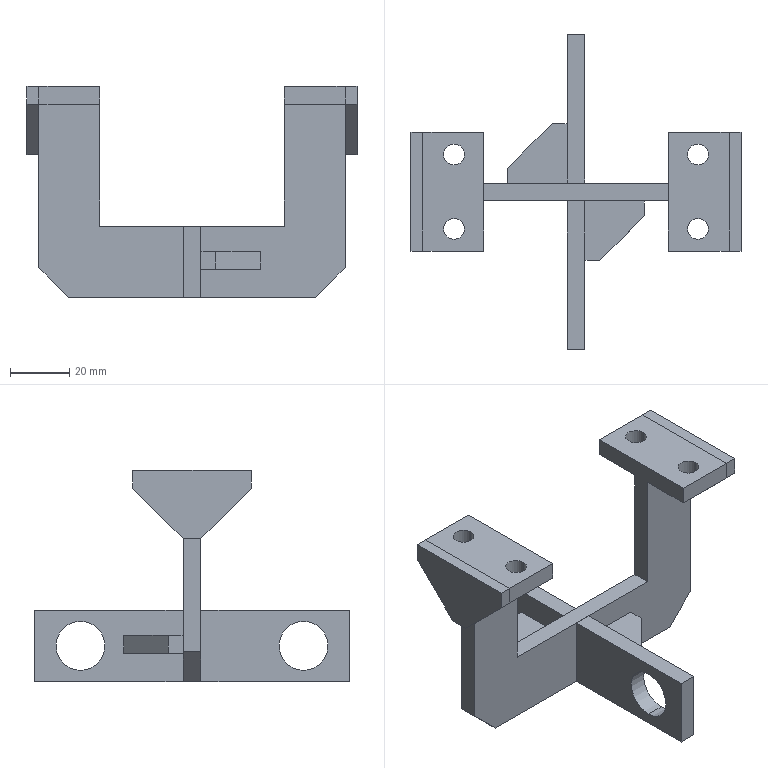Part | SolidWorks | features BaseBody 7 | 7 solids | 74 faces | box 111 x 106 x 71 mm | volume 53566 mm3 | plane 62 | cylinder 12 | commonest cylinder face diameters 7 x8 16.5 x4